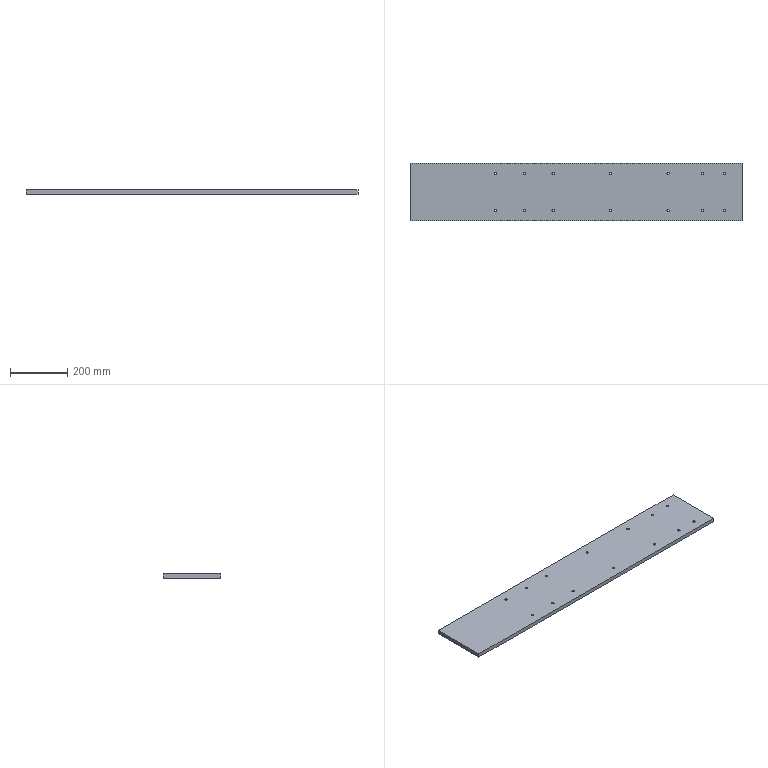Part | STEP file | [06] | 1 solid | 54 faces | box 1155 x 200 x 14 mm | volume 3224487 mm3 | cylinder 36 | plane 10 | cone 8 | commonest cylinder face diameters 8 x28 6 x8